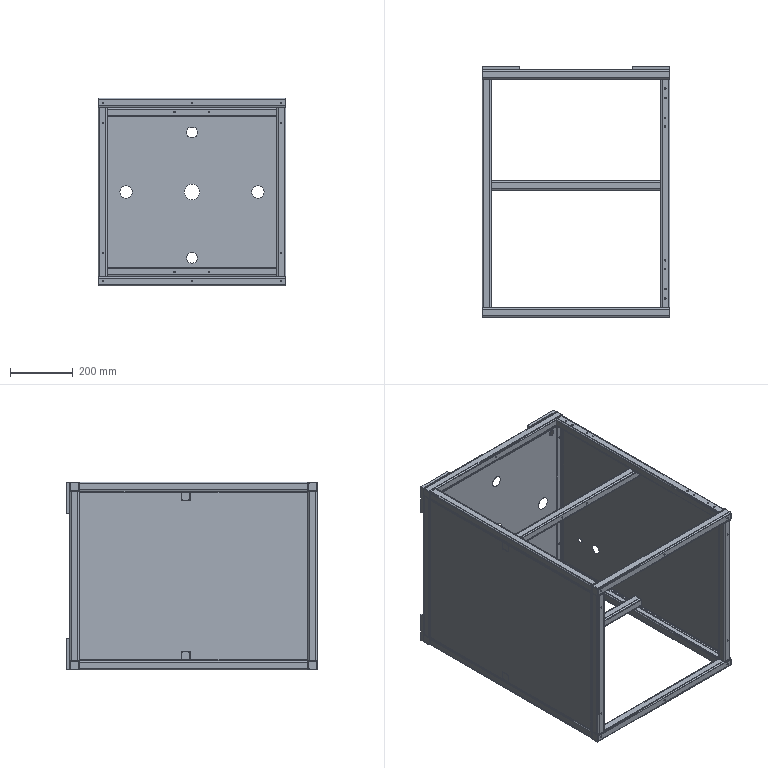Part | SolidWorks | 29 solids | 640 faces | box 600 x 800 x 600 mm | volume 4319374 mm3 | cylinder 350 | plane 290 | commonest cylinder face diameters 4.2 x128 5.2 x56 10.4 x56 5 x32 10 x32 1.473 x8